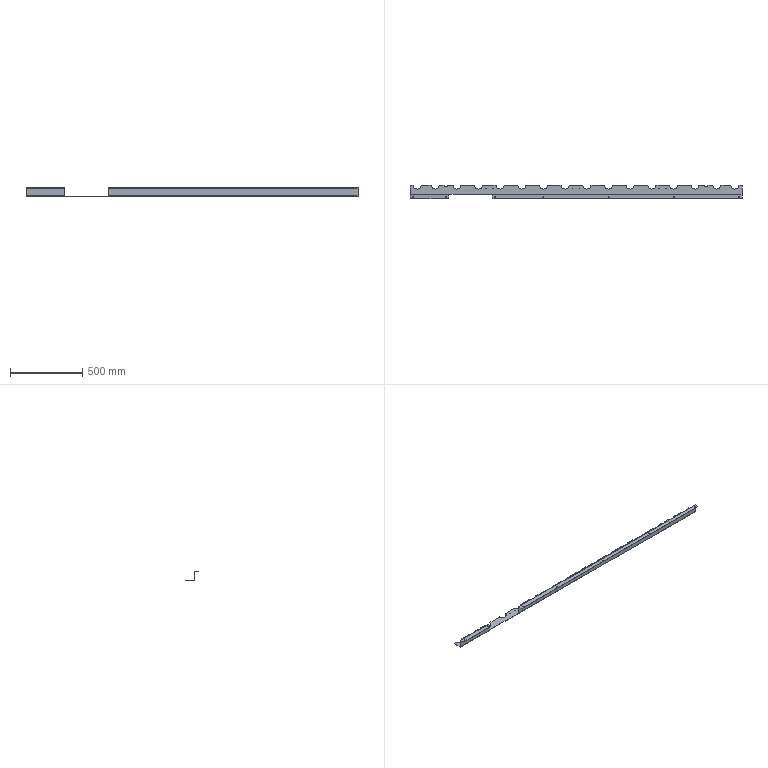Part | STEP file | DCV-000-034-2300L | 1 solid | 188 faces | box 2300 x 94 x 60 mm | volume 480749 mm3 | cylinder 136 | plane 52 | commonest cylinder face diameters 4 x72 54 x16 6 x14 3.242 x12 10 x12 3.2 x4